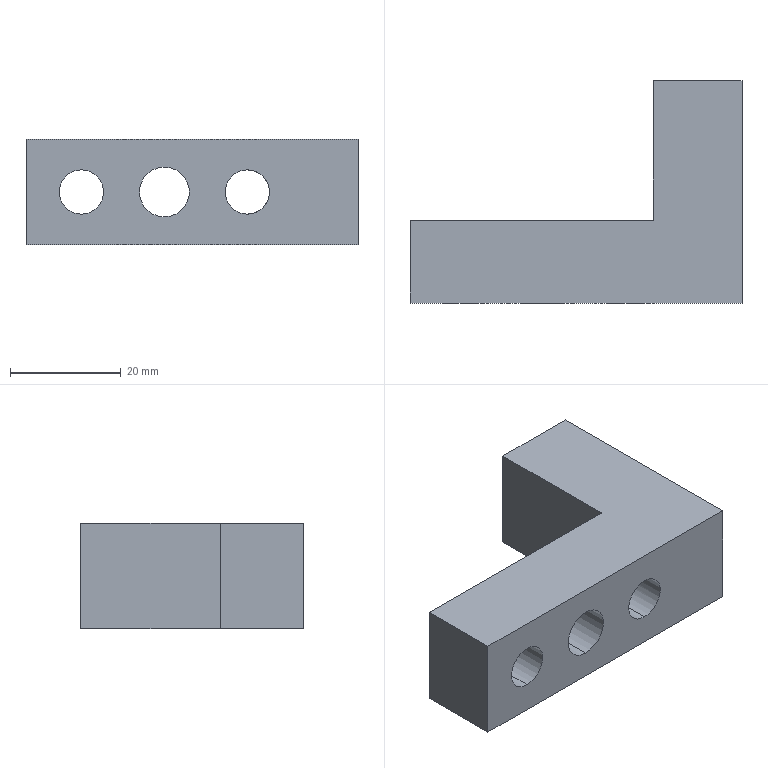Part | SolidWorks | features Extrusion 1, ICE 1 | 1 solid | 14 faces | box 60 x 40.2 x 19 mm | volume 22299 mm3 | plane 8 | cylinder 6 | commonest cylinder face diameters 8 x4 9 x2
STEP:
#1=CARTESIAN_POINT('',(10.,15.,13.5));
#2=VERTEX_POINT('',#1);
#3=CARTESIAN_POINT('',(10.,15.,5.5));
#4=VERTEX_POINT('',#3);
#5=CARTESIAN_POINT('',(10.,15.,9.5));
#6=DIRECTION('',(0.,-1.,0.));
#7=DIRECTION('',(0.,0.,-1.));
#8=AXIS2_PLACEMENT_3D('',#5,#6,#7);
#9=CIRCLE('',#8,4.);
#10=EDGE_CURVE('',#2,#4,#9,.T.);
#11=ORIENTED_EDGE('',*,*,#10,.F.);
#12=CARTESIAN_POINT('',(10.,0.,13.5));
#13=VERTEX_POINT('',#12);
#14=CARTESIAN_POINT('',(10.,15.,13.5));
#15=DIRECTION('',(0.,-1.,0.));
#16=VECTOR('',#15,1000.);
#17=LINE('',#14,#16);
#18=EDGE_CURVE('',#2,#13,#17,.T.);
#19=ORIENTED_EDGE('',*,*,#18,.T.);
#20=CARTESIAN_POINT('',(10.,0.,5.5));
#21=VERTEX_POINT('',#20);
#22=CARTESIAN_POINT('',(10.,0.,9.5));
#23=DIRECTION('',(0.,-1.,0.));
#24=DIRECTION('',(0.,0.,-1.));
#25=AXIS2_PLACEMENT_3D('',#22,#23,#24);
#26=CIRCLE('',#25,4.);
#27=EDGE_CURVE('',#13,#21,#26,.T.);
#28=ORIENTED_EDGE('',*,*,#27,.T.);
#29=CARTESIAN_POINT('',(10.,15.,5.5));
#30=DIRECTION('',(0.,-1.,0.));
#31=VECTOR('',#30,1000.);
#32=LINE('',#29,#31);
#33=EDGE_CURVE('',#4,#21,#32,.T.);
#34=ORIENTED_EDGE('',*,*,#33,.F.);
#35=EDGE_LOOP('',(#11,#19,#28,#34));
#36=FACE_OUTER_BOUND('',#35,.T.);
#37=CARTESIAN_POINT('',(10.,15.,9.5));
#38=DIRECTION('',(0.,-1.,0.));
#39=DIRECTION('',(0.,0.,-1.));
#40=AXIS2_PLACEMENT_3D('',#37,#38,#39);
#41=CYLINDRICAL_SURFACE('',#40,4.);
#42=ADVANCED_FACE('',(#36),#41,.F.);
#43=CARTESIAN_POINT('',(25.,15.,14.));
#44=VERTEX_POINT('',#43);
#45=CARTESIAN_POINT('',(25.,15.,5.));
#46=VERTEX_POINT('',#45);
#47=CARTESIAN_POINT('',(25.,15.,9.5));
#48=DIRECTION('',(0.,-1.,0.));
#49=DIRECTION('',(0.,0.,-1.));
#50=AXIS2_PLACEMENT_3D('',#47,#48,#49);
#51=CIRCLE('',#50,4.5);
#52=EDGE_CURVE('',#44,#46,#51,.T.);
#53=ORIENTED_EDGE('',*,*,#52,.F.);
#54=CARTESIAN_POINT('',(25.,0.,14.));
#55=VERTEX_POINT('',#54);
#56=CARTESIAN_POINT('',(25.,15.,14.));
#57=DIRECTION('',(0.,-1.,0.));
#58=VECTOR('',#57,1000.);
#59=LINE('',#56,#58);
#60=EDGE_CURVE('',#44,#55,#59,.T.);
#61=ORIENTED_EDGE('',*,*,#60,.T.);
#62=CARTESIAN_POINT('',(25.,0.,5.));
#63=VERTEX_POINT('',#62);
#64=CARTESIAN_POINT('',(25.,0.,9.5));
#65=DIRECTION('',(0.,-1.,0.));
#66=DIRECTION('',(0.,0.,-1.));
#67=AXIS2_PLACEMENT_3D('',#64,#65,#66);
#68=CIRCLE('',#67,4.5);
#69=EDGE_CURVE('',#55,#63,#68,.T.);
#70=ORIENTED_EDGE('',*,*,#69,.T.);
#71=CARTESIAN_POINT('',(25.,15.,5.));
#72=DIRECTION('',(0.,-1.,0.));
#73=VECTOR('',#72,1000.);
#74=LINE('',#71,#73);
#75=EDGE_CURVE('',#46,#63,#74,.T.);
#76=ORIENTED_EDGE('',*,*,#75,.F.);
#77=EDGE_LOOP('',(#53,#61,#70,#76));
#78=FACE_OUTER_BOUND('',#77,.T.);
#79=CARTESIAN_POINT('',(25.,15.,9.5));
#80=DIRECTION('',(0.,-1.,0.));
#81=DIRECTION('',(0.,0.,-1.));
#82=AXIS2_PLACEMENT_3D('',#79,#80,#81);
#83=CYLINDRICAL_SURFACE('',#82,4.5);
#84=ADVANCED_FACE('',(#78),#83,.F.);
#85=CARTESIAN_POINT('',(40.,15.,13.5));
#86=VERTEX_POINT('',#85);
#87=CARTESIAN_POINT('',(40.,15.,5.5));
#88=VERTEX_POINT('',#87);
#89=CARTESIAN_POINT('',(40.,15.,9.5));
#90=DIRECTION('',(0.,-1.,0.));
#91=DIRECTION('',(0.,0.,-1.));
#92=AXIS2_PLACEMENT_3D('',#89,#90,#91);
#93=CIRCLE('',#92,4.);
#94=EDGE_CURVE('',#86,#88,#93,.T.);
#95=ORIENTED_EDGE('',*,*,#94,.F.);
#96=CARTESIAN_POINT('',(40.,0.,13.5));
#97=VERTEX_POINT('',#96);
#98=CARTESIAN_POINT('',(40.,15.,13.5));
#99=DIRECTION('',(0.,-1.,0.));
#100=VECTOR('',#99,1000.);
#101=LINE('',#98,#100);
#102=EDGE_CURVE('',#86,#97,#101,.T.);
#103=ORIENTED_EDGE('',*,*,#102,.T.);
#104=CARTESIAN_POINT('',(40.,0.,5.5));
#105=VERTEX_POINT('',#104);
#106=CARTESIAN_POINT('',(40.,0.,9.5));
#107=DIRECTION('',(0.,-1.,0.));
#108=DIRECTION('',(0.,0.,-1.));
#109=AXIS2_PLACEMENT_3D('',#106,#107,#108);
#110=CIRCLE('',#109,4.);
#111=EDGE_CURVE('',#97,#105,#110,.T.);
#112=ORIENTED_EDGE('',*,*,#111,.T.);
#113=CARTESIAN_POINT('',(40.,15.,5.5));
#114=DIRECTION('',(0.,-1.,0.));
#115=VECTOR('',#114,1000.);
#116=LINE('',#113,#115);
#117=EDGE_CURVE('',#88,#105,#116,.T.);
#118=ORIENTED_EDGE('',*,*,#117,.F.);
#119=EDGE_LOOP('',(#95,#103,#112,#118));
#120=FACE_OUTER_BOUND('',#119,.T.);
#121=CARTESIAN_POINT('',(40.,15.,9.5));
#122=DIRECTION('',(0.,-1.,0.));
#123=DIRECTION('',(0.,0.,-1.));
#124=AXIS2_PLACEMENT_3D('',#121,#122,#123);
#125=CYLINDRICAL_SURFACE('',#124,4.);
#126=ADVANCED_FACE('',(#120),#125,.F.);
#127=CARTESIAN_POINT('',(0.,15.,0.));
#128=VERTEX_POINT('',#127);
#129=CARTESIAN_POINT('',(0.,0.,0.));
#130=VERTEX_POINT('',#129);
#131=CARTESIAN_POINT('',(0.,15.,0.));
#132=DIRECTION('',(0.,-1.,0.));
#133=VECTOR('',#132,1000.);
#134=LINE('',#131,#133);
#135=EDGE_CURVE('',#128,#130,#134,.T.);
#136=ORIENTED_EDGE('',*,*,#135,.T.);
#137=CARTESIAN_POINT('',(0.,0.,19.));
#138=VERTEX_POINT('',#137);
#139=CARTESIAN_POINT('',(0.,0.,19.));
#140=DIRECTION('',(0.,0.,-1.));
#141=VECTOR('',#140,1000.);
#142=LINE('',#139,#141);
#143=EDGE_CURVE('',#138,#130,#142,.T.);
#144=ORIENTED_EDGE('',*,*,#143,.F.);
#145=CARTESIAN_POINT('',(0.,15.,19.));
#146=VERTEX_POINT('',#145);
#147=CARTESIAN_POINT('',(0.,15.,19.));
#148=DIRECTION('',(0.,-1.,0.));
#149=VECTOR('',#148,1000.);
#150=LINE('',#147,#149);
#151=EDGE_CURVE('',#146,#138,#150,.T.);
#152=ORIENTED_EDGE('',*,*,#151,.F.);
#153=CARTESIAN_POINT('',(0.,15.,19.));
#154=DIRECTION('',(0.,0.,-1.));
#155=VECTOR('',#154,1000.);
#156=LINE('',#153,#155);
#157=EDGE_CURVE('',#146,#128,#156,.T.);
#158=ORIENTED_EDGE('',*,*,#157,.T.);
#159=EDGE_LOOP('',(#136,#144,#152,#158));
#160=FACE_OUTER_BOUND('',#159,.T.);
#161=CARTESIAN_POINT('',(0.,15.,19.));
#162=DIRECTION('',(1.,0.,0.));
#163=DIRECTION('',(0.,1.,0.));
#164=AXIS2_PLACEMENT_3D('',#161,#162,#163);
#165=PLANE('',#164);
#166=ADVANCED_FACE('',(#160),#165,.F.);
#167=CARTESIAN_POINT('',(10.,0.,9.5));
#168=DIRECTION('',(0.,-1.,0.));
#169=DIRECTION('',(0.,0.,-1.));
#170=AXIS2_PLACEMENT_3D('',#167,#168,#169);
#171=CIRCLE('',#170,4.);
#172=EDGE_CURVE('',#21,#13,#171,.T.);
#173=ORIENTED_EDGE('',*,*,#172,.F.);
#174=ORIENTED_EDGE('',*,*,#27,.F.);
#175=EDGE_LOOP('',(#173,#174));
#176=FACE_BOUND('',#175,.T.);
#177=CARTESIAN_POINT('',(25.,0.,9.5));
#178=DIRECTION('',(0.,-1.,0.));
#179=DIRECTION('',(0.,0.,-1.));
#180=AXIS2_PLACEMENT_3D('',#177,#178,#179);
#181=CIRCLE('',#180,4.5);
#182=EDGE_CURVE('',#63,#55,#181,.T.);
#183=ORIENTED_EDGE('',*,*,#182,.F.);
#184=ORIENTED_EDGE('',*,*,#69,.F.);
#185=EDGE_LOOP('',(#183,#184));
#186=FACE_BOUND('',#185,.T.);
#187=CARTESIAN_POINT('',(40.,0.,9.5));
#188=DIRECTION('',(0.,-1.,0.));
#189=DIRECTION('',(0.,0.,-1.));
#190=AXIS2_PLACEMENT_3D('',#187,#188,#189);
#191=CIRCLE('',#190,4.);
#192=EDGE_CURVE('',#105,#97,#191,.T.);
#193=ORIENTED_EDGE('',*,*,#192,.F.);
#194=ORIENTED_EDGE('',*,*,#111,.F.);
#195=EDGE_LOOP('',(#193,#194));
#196=FACE_BOUND('',#195,.T.);
#197=CARTESIAN_POINT('',(60.,0.,0.));
#198=VERTEX_POINT('',#197);
#199=CARTESIAN_POINT('',(0.,0.,0.));
#200=DIRECTION('',(1.,0.,0.));
#201=VECTOR('',#200,1000.);
#202=LINE('',#199,#201);
#203=EDGE_CURVE('',#130,#198,#202,.T.);
#204=ORIENTED_EDGE('',*,*,#203,.T.);
#205=CARTESIAN_POINT('',(60.,0.,19.));
#206=VERTEX_POINT('',#205);
#207=CARTESIAN_POINT('',(60.,0.,19.));
#208=DIRECTION('',(0.,0.,-1.));
#209=VECTOR('',#208,1000.);
#210=LINE('',#207,#209);
#211=EDGE_CURVE('',#206,#198,#210,.T.);
#212=ORIENTED_EDGE('',*,*,#211,.F.);
#213=CARTESIAN_POINT('',(0.,0.,19.));
#214=DIRECTION('',(1.,0.,0.));
#215=VECTOR('',#214,1000.);
#216=LINE('',#213,#215);
#217=EDGE_CURVE('',#138,#206,#216,.T.);
#218=ORIENTED_EDGE('',*,*,#217,.F.);
#219=ORIENTED_EDGE('',*,*,#143,.T.);
#220=EDGE_LOOP('',(#204,#212,#218,#219));
#221=FACE_OUTER_BOUND('',#220,.T.);
#222=CARTESIAN_POINT('',(0.,0.,19.));
#223=DIRECTION('',(0.,1.,0.));
#224=DIRECTION('',(0.,0.,1.));
#225=AXIS2_PLACEMENT_3D('',#222,#223,#224);
#226=PLANE('',#225);
#227=ADVANCED_FACE('',(#176,#186,#196,#221),#226,.F.);
#228=CARTESIAN_POINT('',(60.,40.2,0.));
#229=VERTEX_POINT('',#228);
#230=CARTESIAN_POINT('',(60.,0.,0.));
#231=DIRECTION('',(0.,1.,0.));
#232=VECTOR('',#231,1000.);
#233=LINE('',#230,#232);
#234=EDGE_CURVE('',#198,#229,#233,.T.);
#235=ORIENTED_EDGE('',*,*,#234,.T.);
#236=CARTESIAN_POINT('',(60.,40.2,19.));
#237=VERTEX_POINT('',#236);
#238=CARTESIAN_POINT('',(60.,40.2,19.));
#239=DIRECTION('',(0.,0.,-1.));
#240=VECTOR('',#239,1000.);
#241=LINE('',#238,#240);
#242=EDGE_CURVE('',#237,#229,#241,.T.);
#243=ORIENTED_EDGE('',*,*,#242,.F.);
#244=CARTESIAN_POINT('',(60.,0.,19.));
#245=DIRECTION('',(0.,1.,0.));
#246=VECTOR('',#245,1000.);
#247=LINE('',#244,#246);
#248=EDGE_CURVE('',#206,#237,#247,.T.);
#249=ORIENTED_EDGE('',*,*,#248,.F.);
#250=ORIENTED_EDGE('',*,*,#211,.T.);
#251=EDGE_LOOP('',(#235,#243,#249,#250));
#252=FACE_OUTER_BOUND('',#251,.T.);
#253=CARTESIAN_POINT('',(60.,0.,19.));
#254=DIRECTION('',(-1.,0.,0.));
#255=DIRECTION('',(0.,0.,1.));
#256=AXIS2_PLACEMENT_3D('',#253,#254,#255);
#257=PLANE('',#256);
#258=ADVANCED_FACE('',(#252),#257,.F.);
#259=CARTESIAN_POINT('',(44.,40.2,0.));
#260=VERTEX_POINT('',#259);
#261=CARTESIAN_POINT('',(60.,40.2,0.));
#262=DIRECTION('',(-1.,0.,0.));
#263=VECTOR('',#262,1000.);
#264=LINE('',#261,#263);
#265=EDGE_CURVE('',#229,#260,#264,.T.);
#266=ORIENTED_EDGE('',*,*,#265,.T.);
#267=CARTESIAN_POINT('',(44.,40.2,19.));
#268=VERTEX_POINT('',#267);
#269=CARTESIAN_POINT('',(44.,40.2,19.));
#270=DIRECTION('',(0.,0.,-1.));
#271=VECTOR('',#270,1000.);
#272=LINE('',#269,#271);
#273=EDGE_CURVE('',#268,#260,#272,.T.);
#274=ORIENTED_EDGE('',*,*,#273,.F.);
#275=CARTESIAN_POINT('',(60.,40.2,19.));
#276=DIRECTION('',(-1.,0.,0.));
#277=VECTOR('',#276,1000.);
#278=LINE('',#275,#277);
#279=EDGE_CURVE('',#237,#268,#278,.T.);
#280=ORIENTED_EDGE('',*,*,#279,.F.);
#281=ORIENTED_EDGE('',*,*,#242,.T.);
#282=EDGE_LOOP('',(#266,#274,#280,#281));
#283=FACE_OUTER_BOUND('',#282,.T.);
#284=CARTESIAN_POINT('',(60.,40.2,19.));
#285=DIRECTION('',(0.,-1.,0.));
#286=DIRECTION('',(0.,0.,-1.));
#287=AXIS2_PLACEMENT_3D('',#284,#285,#286);
#288=PLANE('',#287);
#289=ADVANCED_FACE('',(#283),#288,.F.);
#290=CARTESIAN_POINT('',(44.,15.,0.));
#291=VERTEX_POINT('',#290);
#292=CARTESIAN_POINT('',(44.,40.2,0.));
#293=DIRECTION('',(0.,-1.,0.));
#294=VECTOR('',#293,1000.);
#295=LINE('',#292,#294);
#296=EDGE_CURVE('',#260,#291,#295,.T.);
#297=ORIENTED_EDGE('',*,*,#296,.T.);
#298=CARTESIAN_POINT('',(44.,15.,9.5));
#299=VERTEX_POINT('',#298);
#300=CARTESIAN_POINT('',(44.,15.,19.));
#301=DIRECTION('',(0.,0.,-1.));
#302=VECTOR('',#301,1000.);
#303=LINE('',#300,#302);
#304=EDGE_CURVE('',#299,#291,#303,.T.);
#305=ORIENTED_EDGE('',*,*,#304,.F.);
#306=CARTESIAN_POINT('',(44.,15.,19.));
#307=VERTEX_POINT('',#306);
#308=CARTESIAN_POINT('',(44.,15.,19.));
#309=DIRECTION('',(0.,0.,-1.));
#310=VECTOR('',#309,1000.);
#311=LINE('',#308,#310);
#312=EDGE_CURVE('',#307,#299,#311,.T.);
#313=ORIENTED_EDGE('',*,*,#312,.F.);
#314=CARTESIAN_POINT('',(44.,40.2,19.));
#315=DIRECTION('',(0.,-1.,0.));
#316=VECTOR('',#315,1000.);
#317=LINE('',#314,#316);
#318=EDGE_CURVE('',#268,#307,#317,.T.);
#319=ORIENTED_EDGE('',*,*,#318,.F.);
#320=ORIENTED_EDGE('',*,*,#273,.T.);
#321=EDGE_LOOP('',(#297,#305,#313,#319,#320));
#322=FACE_OUTER_BOUND('',#321,.T.);
#323=CARTESIAN_POINT('',(44.,40.2,19.));
#324=DIRECTION('',(1.,0.,0.));
#325=DIRECTION('',(0.,1.,0.));
#326=AXIS2_PLACEMENT_3D('',#323,#324,#325);
#327=PLANE('',#326);
#328=ADVANCED_FACE('',(#322),#327,.F.);
#329=CARTESIAN_POINT('',(10.,15.,9.5));
#330=DIRECTION('',(0.,-1.,0.));
#331=DIRECTION('',(0.,0.,-1.));
#332=AXIS2_PLACEMENT_3D('',#329,#330,#331);
#333=CIRCLE('',#332,4.);
#334=EDGE_CURVE('',#4,#2,#333,.T.);
#335=ORIENTED_EDGE('',*,*,#334,.T.);
#336=ORIENTED_EDGE('',*,*,#10,.T.);
#337=EDGE_LOOP('',(#335,#336));
#338=FACE_BOUND('',#337,.T.);
#339=CARTESIAN_POINT('',(25.,15.,9.5));
#340=DIRECTION('',(0.,-1.,0.));
#341=DIRECTION('',(0.,0.,-1.));
#342=AXIS2_PLACEMENT_3D('',#339,#340,#341);
#343=CIRCLE('',#342,4.5);
#344=EDGE_CURVE('',#46,#44,#343,.T.);
#345=ORIENTED_EDGE('',*,*,#344,.T.);
#346=ORIENTED_EDGE('',*,*,#52,.T.);
#347=EDGE_LOOP('',(#345,#346));
#348=FACE_BOUND('',#347,.T.);
#349=ORIENTED_EDGE('',*,*,#312,.T.);
#350=CARTESIAN_POINT('',(40.,15.,9.5));
#351=DIRECTION('',(0.,-1.,0.));
#352=DIRECTION('',(0.,0.,-1.));
#353=AXIS2_PLACEMENT_3D('',#350,#351,#352);
#354=CIRCLE('',#353,4.);
#355=EDGE_CURVE('',#299,#86,#354,.T.);
#356=ORIENTED_EDGE('',*,*,#355,.T.);
#357=ORIENTED_EDGE('',*,*,#94,.T.);
#358=CARTESIAN_POINT('',(40.,15.,9.5));
#359=DIRECTION('',(0.,-1.,0.));
#360=DIRECTION('',(0.,0.,-1.));
#361=AXIS2_PLACEMENT_3D('',#358,#359,#360);
#362=CIRCLE('',#361,4.);
#363=EDGE_CURVE('',#88,#299,#362,.T.);
#364=ORIENTED_EDGE('',*,*,#363,.T.);
#365=ORIENTED_EDGE('',*,*,#304,.T.);
#366=CARTESIAN_POINT('',(44.,15.,0.));
#367=DIRECTION('',(-1.,0.,0.));
#368=VECTOR('',#367,1000.);
#369=LINE('',#366,#368);
#370=EDGE_CURVE('',#291,#128,#369,.T.);
#371=ORIENTED_EDGE('',*,*,#370,.T.);
#372=ORIENTED_EDGE('',*,*,#157,.F.);
#373=CARTESIAN_POINT('',(44.,15.,19.));
#374=DIRECTION('',(-1.,0.,0.));
#375=VECTOR('',#374,1000.);
#376=LINE('',#373,#375);
#377=EDGE_CURVE('',#307,#146,#376,.T.);
#378=ORIENTED_EDGE('',*,*,#377,.F.);
#379=EDGE_LOOP('',(#349,#356,#357,#364,#365,#371,#372,#378));
#380=FACE_OUTER_BOUND('',#379,.T.);
#381=CARTESIAN_POINT('',(44.,15.,19.));
#382=DIRECTION('',(0.,-1.,0.));
#383=DIRECTION('',(1.,0.,0.));
#384=AXIS2_PLACEMENT_3D('',#381,#382,#383);
#385=PLANE('',#384);
#386=ADVANCED_FACE('',(#338,#348,#380),#385,.F.);
#387=ORIENTED_EDGE('',*,*,#151,.T.);
#388=ORIENTED_EDGE('',*,*,#217,.T.);
#389=ORIENTED_EDGE('',*,*,#248,.T.);
#390=ORIENTED_EDGE('',*,*,#279,.T.);
#391=ORIENTED_EDGE('',*,*,#318,.T.);
#392=ORIENTED_EDGE('',*,*,#377,.T.);
#393=EDGE_LOOP('',(#387,#388,#389,#390,#391,#392));
#394=FACE_OUTER_BOUND('',#393,.T.);
#395=CARTESIAN_POINT('',(0.,0.,19.));
#396=DIRECTION('',(0.,0.,1.));
#397=DIRECTION('',(1.,0.,0.));
#398=AXIS2_PLACEMENT_3D('',#395,#396,#397);
#399=PLANE('',#398);
#400=ADVANCED_FACE('',(#394),#399,.T.);
#401=ORIENTED_EDGE('',*,*,#135,.F.);
#402=ORIENTED_EDGE('',*,*,#370,.F.);
#403=ORIENTED_EDGE('',*,*,#296,.F.);
#404=ORIENTED_EDGE('',*,*,#265,.F.);
#405=ORIENTED_EDGE('',*,*,#234,.F.);
#406=ORIENTED_EDGE('',*,*,#203,.F.);
#407=EDGE_LOOP('',(#401,#402,#403,#404,#405,#406));
#408=FACE_OUTER_BOUND('',#407,.T.);
#409=CARTESIAN_POINT('',(0.,0.,0.));
#410=DIRECTION('',(0.,0.,1.));
#411=DIRECTION('',(1.,0.,0.));
#412=AXIS2_PLACEMENT_3D('',#409,#410,#411);
#413=PLANE('',#412);
#414=ADVANCED_FACE('',(#408),#413,.F.);
#415=ORIENTED_EDGE('',*,*,#102,.F.);
#416=ORIENTED_EDGE('',*,*,#355,.F.);
#417=ORIENTED_EDGE('',*,*,#363,.F.);
#418=ORIENTED_EDGE('',*,*,#117,.T.);
#419=ORIENTED_EDGE('',*,*,#192,.T.);
#420=EDGE_LOOP('',(#415,#416,#417,#418,#419));
#421=FACE_OUTER_BOUND('',#420,.T.);
#422=CARTESIAN_POINT('',(40.,15.,9.5));
#423=DIRECTION('',(0.,-1.,0.));
#424=DIRECTION('',(0.,0.,-1.));
#425=AXIS2_PLACEMENT_3D('',#422,#423,#424);
#426=CYLINDRICAL_SURFACE('',#425,4.);
#427=ADVANCED_FACE('',(#421),#426,.F.);
#428=ORIENTED_EDGE('',*,*,#60,.F.);
#429=ORIENTED_EDGE('',*,*,#344,.F.);
#430=ORIENTED_EDGE('',*,*,#75,.T.);
#431=ORIENTED_EDGE('',*,*,#182,.T.);
#432=EDGE_LOOP('',(#428,#429,#430,#431));
#433=FACE_OUTER_BOUND('',#432,.T.);
#434=CARTESIAN_POINT('',(25.,15.,9.5));
#435=DIRECTION('',(0.,-1.,0.));
#436=DIRECTION('',(0.,0.,-1.));
#437=AXIS2_PLACEMENT_3D('',#434,#435,#436);
#438=CYLINDRICAL_SURFACE('',#437,4.5);
#439=ADVANCED_FACE('',(#433),#438,.F.);
#440=ORIENTED_EDGE('',*,*,#18,.F.);
#441=ORIENTED_EDGE('',*,*,#334,.F.);
#442=ORIENTED_EDGE('',*,*,#33,.T.);
#443=ORIENTED_EDGE('',*,*,#172,.T.);
#444=EDGE_LOOP('',(#440,#441,#442,#443));
#445=FACE_OUTER_BOUND('',#444,.T.);
#446=CARTESIAN_POINT('',(10.,15.,9.5));
#447=DIRECTION('',(0.,-1.,0.));
#448=DIRECTION('',(0.,0.,-1.));
#449=AXIS2_PLACEMENT_3D('',#446,#447,#448);
#450=CYLINDRICAL_SURFACE('',#449,4.);
#451=ADVANCED_FACE('',(#445),#450,.F.);
#452=CLOSED_SHELL('',(#42,#84,#126,#166,#227,#258,#289,#328,#386,#400,#414,#427,#439,#451));
#453=MANIFOLD_SOLID_BREP('',#452);
#454=CARTESIAN_POINT('',(0.,0.,0.));
#455=DIRECTION('',(0.,0.,1.));
#456=DIRECTION('',(1.,0.,0.));
#457=AXIS2_PLACEMENT_3D('',#454,#455,#456);
#458=(LENGTH_UNIT()NAMED_UNIT(*)SI_UNIT(.MILLI.,.METRE.));
#459=UNCERTAINTY_MEASURE_WITH_UNIT(LENGTH_MEASURE(0.00001),#458,'','');
#460=(NAMED_UNIT(*)PLANE_ANGLE_UNIT()SI_UNIT($,.RADIAN.));
#461=(NAMED_UNIT(*)SI_UNIT($,.STERADIAN.)SOLID_ANGLE_UNIT());
#462=(GEOMETRIC_REPRESENTATION_CONTEXT(3)GLOBAL_UNCERTAINTY_ASSIGNED_CONTEXT((#459))GLOBAL_UNIT_ASSIGNED_CONTEXT((#458,#460,#461))REPRESENTATION_CONTEXT('',''));
#463=ADVANCED_BREP_SHAPE_REPRESENTATION('',(#453,#457),#462);